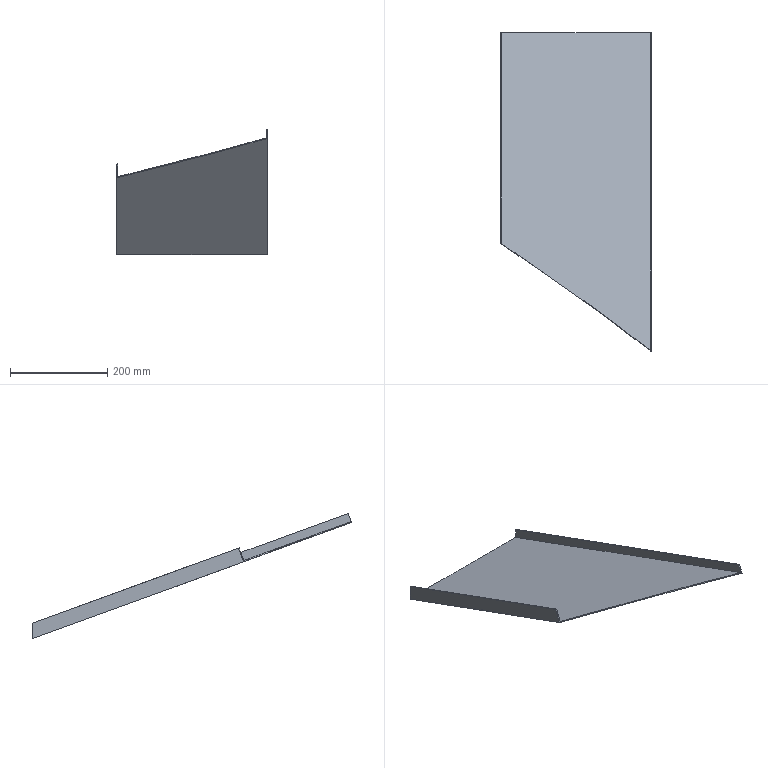Part | NX | features solid 2 | 1 solid | 11 faces | box 310 x 657.989 x 258.282 mm | volume 406239 mm3 | plane 10 | spline 1
STEP:
#1=CARTESIAN_POINT('',(513.,524.25,-139.857));
#2=VERTEX_POINT('',#1);
#3=CARTESIAN_POINT('',(513.,1180.,-378.53));
#4=VERTEX_POINT('',#3);
#5=CARTESIAN_POINT('',(513.,1053.844,-332.613));
#6=DIRECTION('',(0.,0.9397,-0.342));
#7=VECTOR('',#6,1000.);
#8=LINE('',#5,#7);
#9=EDGE_CURVE('',#2,#4,#8,.T.);
#10=ORIENTED_EDGE('',*,*,#9,.T.);
#11=CARTESIAN_POINT('',(207.,1180.,-378.53));
#12=VERTEX_POINT('',#11);
#13=CARTESIAN_POINT('',(-675.,1180.,-378.53));
#14=DIRECTION('',(-1.,0.,0.));
#15=VECTOR('',#14,1000.);
#16=LINE('',#13,#15);
#17=EDGE_CURVE('',#12,#4,#16,.F.);
#18=ORIENTED_EDGE('',*,*,#17,.F.);
#19=CARTESIAN_POINT('',(207.,744.184,-219.906));
#20=VERTEX_POINT('',#19);
#21=CARTESIAN_POINT('',(207.,1053.844,-332.613));
#22=DIRECTION('',(0.,0.9397,-0.342));
#23=VECTOR('',#22,1000.);
#24=LINE('',#21,#23);
#25=EDGE_CURVE('',#20,#12,#24,.T.);
#26=ORIENTED_EDGE('',*,*,#25,.F.);
#27=CARTESIAN_POINT('',(270.,700.581,-204.036));
#28=VERTEX_POINT('',#27);
#29=CARTESIAN_POINT('',(202.195,747.51,-221.116));
#30=CARTESIAN_POINT('',(270.081,700.526,-204.015));
#31=CARTESIAN_POINT('',(337.967,653.541,-186.914));
#32=CARTESIAN_POINT('',(342.606,650.33,-185.746));
#33=CARTESIAN_POINT('',(357.056,640.2,-182.059));
#34=CARTESIAN_POINT('',(366.847,633.337,-179.561));
#35=CARTESIAN_POINT('',(376.081,626.783,-177.175));
#36=CARTESIAN_POINT('',(395.621,612.917,-172.128));
#37=CARTESIAN_POINT('',(413.842,599.597,-167.281));
#38=CARTESIAN_POINT('',(451.399,572.143,-157.288));
#39=CARTESIAN_POINT('',(488.058,543.642,-146.914));
#40=CARTESIAN_POINT('',(518.274,520.15,-138.364));
#41=CARTESIAN_POINT('',(548.491,496.657,-129.813));
#42=CARTESIAN_POINT('',(578.708,473.165,-121.263));
#43=CARTESIAN_POINT('',(608.924,449.673,-112.712));
#44=CARTESIAN_POINT('',(639.141,426.18,-104.162));
#45=CARTESIAN_POINT('',(669.357,402.688,-95.611));
#46=CARTESIAN_POINT('',(699.574,379.196,-87.061));
#47=CARTESIAN_POINT('',(729.79,355.703,-78.51));
#48=B_SPLINE_CURVE_WITH_KNOTS('',2,(#29,#30,#31,#32,#33,#34,#35,#36,#37,#38,#39,#40,#41,#42,#43,#44,#45,#46,#47),.UNSPECIFIED.,.F.,.F.,(3,2,2,2,2,2,2,2,2,3),(-1.829,0.,0.125,0.25,0.5,1.,1.412,1.824,2.236,2.649),.PIECEWISE_BEZIER_KNOTS.);
#49=EDGE_CURVE('',#20,#28,#48,.T.);
#50=ORIENTED_EDGE('',*,*,#49,.T.);
#51=CARTESIAN_POINT('',(513.,524.25,-139.857));
#52=CARTESIAN_POINT('',(503.143,531.914,-142.646));
#53=CARTESIAN_POINT('',(483.463,547.283,-148.24));
#54=CARTESIAN_POINT('',(443.791,577.659,-159.296));
#55=CARTESIAN_POINT('',(393.431,614.763,-172.801));
#56=CARTESIAN_POINT('',(331.874,657.869,-188.49));
#57=CARTESIAN_POINT('',(290.605,686.32,-198.845));
#58=CARTESIAN_POINT('',(270.,700.581,-204.036));
#59=B_SPLINE_CURVE_WITH_KNOTS('',3,(#51,#52,#53,#54,#55,#56,#57,#58),.UNSPECIFIED.,.F.,.F.,(4,1,1,1,1,4),(0.525,0.5634,0.6018,0.6786,0.7553,0.8321),.UNSPECIFIED.);
#60=EDGE_CURVE('',#28,#2,#59,.F.);
#61=ORIENTED_EDGE('',*,*,#60,.T.);
#62=EDGE_LOOP('',(#10,#18,#26,#50,#61));
#63=FACE_BOUND('',#62,.T.);
#64=CARTESIAN_POINT('',(920.,1053.844,-332.613));
#65=DIRECTION('',(0.,0.342,0.9397));
#66=DIRECTION('',(0.,-0.9397,0.342));
#67=AXIS2_PLACEMENT_3D('',#64,#65,#66);
#68=PLANE('',#67);
#69=ADVANCED_FACE('',(#63),#68,.T.);
#70=CARTESIAN_POINT('',(205.,744.885,-222.289));
#71=VERTEX_POINT('',#70);
#72=CARTESIAN_POINT('',(205.,1180.,-380.658));
#73=VERTEX_POINT('',#72);
#74=CARTESIAN_POINT('',(205.,991.87,-312.185));
#75=DIRECTION('',(0.,0.9397,-0.342));
#76=VECTOR('',#75,1000.);
#77=LINE('',#74,#76);
#78=EDGE_CURVE('',#71,#73,#77,.T.);
#79=ORIENTED_EDGE('',*,*,#78,.F.);
#80=CARTESIAN_POINT('',(205.,755.145,-194.098));
#81=VERTEX_POINT('',#80);
#82=CARTESIAN_POINT('',(205.,755.145,-194.098));
#83=DIRECTION('',(0.,-0.342,-0.9397));
#84=VECTOR('',#83,1000.);
#85=LINE('',#82,#84);
#86=EDGE_CURVE('',#81,#71,#85,.T.);
#87=ORIENTED_EDGE('',*,*,#86,.F.);
#88=CARTESIAN_POINT('',(205.,1180.,-348.733));
#89=VERTEX_POINT('',#88);
#90=CARTESIAN_POINT('',(205.,1002.131,-283.994));
#91=DIRECTION('',(0.,-0.9397,0.342));
#92=VECTOR('',#91,1000.);
#93=LINE('',#90,#92);
#94=EDGE_CURVE('',#81,#89,#93,.F.);
#95=ORIENTED_EDGE('',*,*,#94,.T.);
#96=CARTESIAN_POINT('',(205.,1180.,-730.));
#97=DIRECTION('',(0.,0.,-1.));
#98=VECTOR('',#97,1000.);
#99=LINE('',#96,#98);
#100=EDGE_CURVE('',#73,#89,#99,.F.);
#101=ORIENTED_EDGE('',*,*,#100,.F.);
#102=EDGE_LOOP('',(#79,#87,#95,#101));
#103=FACE_BOUND('',#102,.T.);
#104=CARTESIAN_POINT('',(205.,999.395,-291.511));
#105=DIRECTION('',(-1.,0.,0.));
#106=DIRECTION('',(0.,-1.,0.));
#107=AXIS2_PLACEMENT_3D('',#104,#105,#106);
#108=PLANE('',#107);
#109=ADVANCED_FACE('',(#103),#108,.T.);
#110=CARTESIAN_POINT('',(513.,523.566,-141.736));
#111=VERTEX_POINT('',#110);
#112=CARTESIAN_POINT('',(513.,523.566,-141.736));
#113=CARTESIAN_POINT('',(500.551,533.245,-145.259));
#114=CARTESIAN_POINT('',(475.704,552.661,-152.326));
#115=CARTESIAN_POINT('',(425.39,590.785,-166.202));
#116=CARTESIAN_POINT('',(374.104,627.774,-179.665));
#117=CARTESIAN_POINT('',(322.106,663.848,-192.794));
#118=CARTESIAN_POINT('',(270.051,699.855,-205.9));
#119=CARTESIAN_POINT('',(231.022,726.875,-215.734));
#120=CARTESIAN_POINT('',(205.,744.885,-222.289));
#121=B_SPLINE_CURVE_WITH_KNOTS('',3,(#112,#113,#114,#115,#116,#117,#118,#119,#120),.UNSPECIFIED.,.F.,.F.,(4,1,1,1,1,1,4),(1.817,1.865,1.914,2.01,2.059,2.107,2.204),.UNSPECIFIED.);
#122=EDGE_CURVE('',#71,#111,#121,.F.);
#123=ORIENTED_EDGE('',*,*,#122,.F.);
#124=ORIENTED_EDGE('',*,*,#78,.T.);
#125=CARTESIAN_POINT('',(515.,1180.,-380.658));
#126=VERTEX_POINT('',#125);
#127=CARTESIAN_POINT('',(-675.,1180.,-380.658));
#128=DIRECTION('',(-1.,0.,0.));
#129=VECTOR('',#128,1000.);
#130=LINE('',#127,#129);
#131=EDGE_CURVE('',#73,#126,#130,.F.);
#132=ORIENTED_EDGE('',*,*,#131,.T.);
#133=CARTESIAN_POINT('',(515.,522.011,-141.17));
#134=VERTEX_POINT('',#133);
#135=CARTESIAN_POINT('',(515.,1053.16,-334.492));
#136=DIRECTION('',(0.,0.9397,-0.342));
#137=VECTOR('',#136,1000.);
#138=LINE('',#135,#137);
#139=EDGE_CURVE('',#134,#126,#138,.T.);
#140=ORIENTED_EDGE('',*,*,#139,.F.);
#141=CARTESIAN_POINT('',(513.,522.011,-141.17));
#142=VERTEX_POINT('',#141);
#143=CARTESIAN_POINT('',(515.,522.011,-141.17));
#144=DIRECTION('',(-1.,0.,0.));
#145=VECTOR('',#144,1000.);
#146=LINE('',#143,#145);
#147=EDGE_CURVE('',#134,#142,#146,.T.);
#148=ORIENTED_EDGE('',*,*,#147,.T.);
#149=CARTESIAN_POINT('',(513.,522.011,-141.17));
#150=DIRECTION('',(0.,0.9397,-0.342));
#151=VECTOR('',#150,1000.);
#152=LINE('',#149,#151);
#153=EDGE_CURVE('',#142,#111,#152,.T.);
#154=ORIENTED_EDGE('',*,*,#153,.T.);
#155=EDGE_LOOP('',(#123,#124,#132,#140,#148,#154));
#156=FACE_BOUND('',#155,.T.);
#157=CARTESIAN_POINT('',(920.,1053.16,-334.492));
#158=DIRECTION('',(0.,0.342,0.9397));
#159=DIRECTION('',(0.,-0.9397,0.342));
#160=AXIS2_PLACEMENT_3D('',#157,#158,#159);
#161=PLANE('',#160);
#162=ADVANCED_FACE('',(#156),#161,.F.);
#163=ORIENTED_EDGE('',*,*,#94,.F.);
#164=CARTESIAN_POINT('',(207.,753.761,-193.595));
#165=VERTEX_POINT('',#164);
#166=CARTESIAN_POINT('',(207.,753.761,-193.595));
#167=CARTESIAN_POINT('',(206.333,754.222,-193.763));
#168=CARTESIAN_POINT('',(205.667,754.684,-193.931));
#169=CARTESIAN_POINT('',(205.,755.145,-194.098));
#170=B_SPLINE_CURVE_WITH_KNOTS('',3,(#166,#167,#168,#169),.UNSPECIFIED.,.F.,.F.,(4,4),(0.07824,0.08073),.UNSPECIFIED.);
#171=EDGE_CURVE('',#165,#81,#170,.T.);
#172=ORIENTED_EDGE('',*,*,#171,.F.);
#173=CARTESIAN_POINT('',(207.,1180.,-348.733));
#174=VERTEX_POINT('',#173);
#175=CARTESIAN_POINT('',(207.,710.158,-177.724));
#176=DIRECTION('',(0.,-0.9397,0.342));
#177=VECTOR('',#176,1000.);
#178=LINE('',#175,#177);
#179=EDGE_CURVE('',#165,#174,#178,.F.);
#180=ORIENTED_EDGE('',*,*,#179,.T.);
#181=CARTESIAN_POINT('',(-675.,1180.,-348.733));
#182=DIRECTION('',(1.,0.,0.));
#183=VECTOR('',#182,1000.);
#184=LINE('',#181,#183);
#185=EDGE_CURVE('',#89,#174,#184,.T.);
#186=ORIENTED_EDGE('',*,*,#185,.F.);
#187=EDGE_LOOP('',(#163,#172,#180,#186));
#188=FACE_BOUND('',#187,.T.);
#189=CARTESIAN_POINT('',(270.,710.158,-177.724));
#190=DIRECTION('',(0.,-0.342,-0.9397));
#191=DIRECTION('',(0.,0.9397,-0.342));
#192=AXIS2_PLACEMENT_3D('',#189,#190,#191);
#193=PLANE('',#192);
#194=ADVANCED_FACE('',(#188),#193,.F.);
#195=ORIENTED_EDGE('',*,*,#25,.T.);
#196=CARTESIAN_POINT('',(207.,1180.,-730.));
#197=DIRECTION('',(0.,0.,1.));
#198=VECTOR('',#197,1000.);
#199=LINE('',#196,#198);
#200=EDGE_CURVE('',#174,#12,#199,.F.);
#201=ORIENTED_EDGE('',*,*,#200,.F.);
#202=ORIENTED_EDGE('',*,*,#179,.F.);
#203=CARTESIAN_POINT('',(207.,748.973,-206.75));
#204=DIRECTION('',(0.,-0.342,-0.9397));
#205=VECTOR('',#204,1000.);
#206=LINE('',#203,#205);
#207=EDGE_CURVE('',#20,#165,#206,.F.);
#208=ORIENTED_EDGE('',*,*,#207,.F.);
#209=EDGE_LOOP('',(#195,#201,#202,#208));
#210=FACE_BOUND('',#209,.T.);
#211=CARTESIAN_POINT('',(207.,706.738,-187.121));
#212=DIRECTION('',(1.,0.,0.));
#213=DIRECTION('',(0.,1.,0.));
#214=AXIS2_PLACEMENT_3D('',#211,#212,#213);
#215=PLANE('',#214);
#216=ADVANCED_FACE('',(#210),#215,.T.);
#217=ORIENTED_EDGE('',*,*,#60,.F.);
#218=ORIENTED_EDGE('',*,*,#49,.F.);
#219=ORIENTED_EDGE('',*,*,#207,.T.);
#220=ORIENTED_EDGE('',*,*,#171,.T.);
#221=ORIENTED_EDGE('',*,*,#86,.T.);
#222=ORIENTED_EDGE('',*,*,#122,.T.);
#223=CARTESIAN_POINT('',(513.,531.091,-121.063));
#224=DIRECTION('',(0.,-0.342,-0.9397));
#225=VECTOR('',#224,1000.);
#226=LINE('',#223,#225);
#227=EDGE_CURVE('',#2,#111,#226,.T.);
#228=ORIENTED_EDGE('',*,*,#227,.F.);
#229=EDGE_LOOP('',(#217,#218,#219,#220,#221,#222,#228));
#230=FACE_BOUND('',#229,.T.);
#231=CARTESIAN_POINT('',(205.,755.145,-194.098));
#232=CARTESIAN_POINT('',(205.,744.885,-222.289));
#233=CARTESIAN_POINT('',(223.318,742.467,-189.484));
#234=CARTESIAN_POINT('',(223.318,732.206,-217.675));
#235=CARTESIAN_POINT('',(246.217,726.619,-183.716));
#236=CARTESIAN_POINT('',(246.217,716.358,-211.906));
#237=CARTESIAN_POINT('',(273.694,707.601,-176.794));
#238=CARTESIAN_POINT('',(273.694,697.341,-204.985));
#239=CARTESIAN_POINT('',(287.433,698.092,-173.333));
#240=CARTESIAN_POINT('',(287.433,687.832,-201.524));
#241=CARTESIAN_POINT('',(298.882,690.168,-170.449));
#242=CARTESIAN_POINT('',(298.882,679.908,-198.64));
#243=CARTESIAN_POINT('',(308.042,683.829,-168.141));
#244=CARTESIAN_POINT('',(308.042,673.568,-196.332));
#245=CARTESIAN_POINT('',(314.911,679.075,-166.411));
#246=CARTESIAN_POINT('',(314.911,668.814,-194.602));
#247=CARTESIAN_POINT('',(321.781,674.32,-164.68));
#248=CARTESIAN_POINT('',(321.781,664.06,-192.871));
#249=CARTESIAN_POINT('',(327.504,670.359,-163.239));
#250=CARTESIAN_POINT('',(327.504,660.098,-191.429));
#251=CARTESIAN_POINT('',(332.085,667.188,-162.085));
#252=CARTESIAN_POINT('',(332.085,656.927,-190.275));
#253=CARTESIAN_POINT('',(334.944,665.209,-161.364));
#254=CARTESIAN_POINT('',(334.944,654.949,-189.555));
#255=CARTESIAN_POINT('',(337.241,663.62,-160.786));
#256=CARTESIAN_POINT('',(337.241,653.359,-188.977));
#257=CARTESIAN_POINT('',(338.938,662.445,-160.358));
#258=CARTESIAN_POINT('',(338.938,652.185,-188.549));
#259=CARTESIAN_POINT('',(341.397,660.734,-159.736));
#260=CARTESIAN_POINT('',(341.397,650.473,-187.926));
#261=CARTESIAN_POINT('',(344.504,658.565,-158.946));
#262=CARTESIAN_POINT('',(344.504,648.304,-187.137));
#263=CARTESIAN_POINT('',(348.288,655.919,-157.983));
#264=CARTESIAN_POINT('',(348.288,645.659,-186.174));
#265=CARTESIAN_POINT('',(352.007,653.315,-157.035));
#266=CARTESIAN_POINT('',(352.007,643.055,-185.226));
#267=CARTESIAN_POINT('',(354.685,651.439,-156.352));
#268=CARTESIAN_POINT('',(354.685,641.178,-184.543));
#269=CARTESIAN_POINT('',(355.986,650.527,-156.02));
#270=CARTESIAN_POINT('',(355.986,640.266,-184.211));
#271=CARTESIAN_POINT('',(356.517,650.154,-155.885));
#272=CARTESIAN_POINT('',(356.517,639.894,-184.076));
#273=CARTESIAN_POINT('',(356.994,649.821,-155.763));
#274=CARTESIAN_POINT('',(356.994,639.56,-183.954));
#275=CARTESIAN_POINT('',(357.305,649.602,-155.684));
#276=CARTESIAN_POINT('',(357.305,639.342,-183.875));
#277=CARTESIAN_POINT('',(357.827,649.236,-155.551));
#278=CARTESIAN_POINT('',(357.827,638.976,-183.741));
#279=CARTESIAN_POINT('',(358.583,648.706,-155.358));
#280=CARTESIAN_POINT('',(358.583,638.445,-183.548));
#281=CARTESIAN_POINT('',(359.783,647.864,-155.051));
#282=CARTESIAN_POINT('',(359.783,637.603,-183.242));
#283=CARTESIAN_POINT('',(361.279,646.813,-154.669));
#284=CARTESIAN_POINT('',(361.279,636.552,-182.859));
#285=CARTESIAN_POINT('',(363.064,645.558,-154.212));
#286=CARTESIAN_POINT('',(363.064,635.297,-182.403));
#287=CARTESIAN_POINT('',(365.432,643.891,-153.605));
#288=CARTESIAN_POINT('',(365.432,633.63,-181.796));
#289=CARTESIAN_POINT('',(368.365,641.823,-152.852));
#290=CARTESIAN_POINT('',(368.365,631.562,-181.043));
#291=CARTESIAN_POINT('',(371.86,639.352,-151.953));
#292=CARTESIAN_POINT('',(371.86,629.092,-180.144));
#293=CARTESIAN_POINT('',(374.698,637.341,-151.221));
#294=CARTESIAN_POINT('',(374.698,627.081,-179.412));
#295=CARTESIAN_POINT('',(377.045,635.676,-150.615));
#296=CARTESIAN_POINT('',(377.045,625.415,-178.806));
#297=CARTESIAN_POINT('',(379.464,633.957,-149.99));
#298=CARTESIAN_POINT('',(379.464,623.697,-178.18));
#299=CARTESIAN_POINT('',(383.64,630.984,-148.907));
#300=CARTESIAN_POINT('',(383.64,620.723,-177.098));
#301=CARTESIAN_POINT('',(389.569,626.746,-147.365));
#302=CARTESIAN_POINT('',(389.569,616.485,-175.556));
#303=CARTESIAN_POINT('',(396.586,621.702,-145.529));
#304=CARTESIAN_POINT('',(396.586,611.441,-173.72));
#305=CARTESIAN_POINT('',(403.507,616.701,-143.709));
#306=CARTESIAN_POINT('',(403.507,606.44,-171.899));
#307=CARTESIAN_POINT('',(409.227,612.544,-142.196));
#308=CARTESIAN_POINT('',(409.227,602.283,-170.387));
#309=CARTESIAN_POINT('',(413.694,609.283,-141.009));
#310=CARTESIAN_POINT('',(413.694,599.022,-169.2));
#311=CARTESIAN_POINT('',(418.36,605.868,-139.766));
#312=CARTESIAN_POINT('',(418.36,595.607,-167.957));
#313=CARTESIAN_POINT('',(424.124,601.631,-138.224));
#314=CARTESIAN_POINT('',(424.124,591.37,-166.414));
#315=CARTESIAN_POINT('',(437.974,591.39,-134.496));
#316=CARTESIAN_POINT('',(437.974,581.129,-162.687));
#317=CARTESIAN_POINT('',(458.619,575.914,-128.864));
#318=CARTESIAN_POINT('',(458.619,565.653,-157.054));
#319=CARTESIAN_POINT('',(485.887,554.958,-121.236));
#320=CARTESIAN_POINT('',(485.887,544.698,-149.427));
#321=CARTESIAN_POINT('',(503.953,540.86,-116.105));
#322=CARTESIAN_POINT('',(503.953,530.6,-144.296));
#323=CARTESIAN_POINT('',(513.,533.827,-113.545));
#324=CARTESIAN_POINT('',(513.,523.566,-141.736));
#325=B_SPLINE_SURFACE_WITH_KNOTS('',3,1,((#231,#232),(#233,#234),(#235,#236),(#237,#238),(#239,#240),(#241,#242),(#243,#244),(#245,#246),(#247,#248),(#249,#250),(#251,#252),(#253,#254),(#255,#256),(#257,#258),(#259,#260),(#261,#262),(#263,#264),(#265,#266),(#267,#268),(#269,#270),(#271,#272),(#273,#274),(#275,#276),(#277,#278),(#279,#280),(#281,#282),(#283,#284),(#285,#286),(#287,#288),(#289,#290),(#291,#292),(#293,#294),(#295,#296),(#297,#298),(#299,#300),(#301,#302),(#303,#304),(#305,#306),(#307,#308),(#309,#310),(#311,#312),(#313,#314),(#315,#316),(#317,#318),(#319,#320),(#321,#322),(#323,#324)),.UNSPECIFIED.,.F.,.F.,.F.,(4,1,1,1,1,1,1,1,1,1,1,1,1,1,1,1,1,1,1,1,1,1,1,1,1,1,1,1,1,1,1,1,1,1,1,1,1,1,1,1,1,1,1,1,4),(2,2),(-1.791,-1.051,-0.8659,-0.6808,-0.4957,-0.4031,-0.3106,-0.2181,-0.1255,-0.07924,-0.03297,-0.009836,0.0133,0.03644,0.05957,0.08271,0.1058,0.1174,0.1203,0.1232,0.1246,0.1261,0.129,0.1348,0.1405,0.1521,0.1637,0.1753,0.1984,0.2215,0.2447,0.2562,0.2678,0.2909,0.3372,0.3835,0.4297,0.476,0.4992,0.5223,0.5686,0.6148,0.7999,0.985,1.17),(0.,1.),.UNSPECIFIED.);
#326=ADVANCED_FACE('',(#230),#325,.F.);
#327=ORIENTED_EDGE('',*,*,#17,.T.);
#328=CARTESIAN_POINT('',(513.,1180.,-359.375));
#329=VERTEX_POINT('',#328);
#330=CARTESIAN_POINT('',(513.,1180.,-730.));
#331=DIRECTION('',(0.,0.,-1.));
#332=VECTOR('',#331,1000.);
#333=LINE('',#330,#332);
#334=EDGE_CURVE('',#4,#329,#333,.F.);
#335=ORIENTED_EDGE('',*,*,#334,.T.);
#336=CARTESIAN_POINT('',(515.,1180.,-359.375));
#337=VERTEX_POINT('',#336);
#338=CARTESIAN_POINT('',(515.,1180.,-359.375));
#339=DIRECTION('',(-1.,0.,0.));
#340=VECTOR('',#339,1000.);
#341=LINE('',#338,#340);
#342=EDGE_CURVE('',#337,#329,#341,.T.);
#343=ORIENTED_EDGE('',*,*,#342,.F.);
#344=CARTESIAN_POINT('',(515.,1180.,-730.));
#345=DIRECTION('',(0.,0.,-1.));
#346=VECTOR('',#345,1000.);
#347=LINE('',#344,#346);
#348=EDGE_CURVE('',#126,#337,#347,.F.);
#349=ORIENTED_EDGE('',*,*,#348,.F.);
#350=ORIENTED_EDGE('',*,*,#131,.F.);
#351=ORIENTED_EDGE('',*,*,#100,.T.);
#352=ORIENTED_EDGE('',*,*,#185,.T.);
#353=ORIENTED_EDGE('',*,*,#200,.T.);
#354=EDGE_LOOP('',(#327,#335,#343,#349,#350,#351,#352,#353));
#355=FACE_BOUND('',#354,.T.);
#356=CARTESIAN_POINT('',(-675.,1180.,-730.));
#357=DIRECTION('',(0.,-1.,0.));
#358=DIRECTION('',(1.,0.,0.));
#359=AXIS2_PLACEMENT_3D('',#356,#357,#358);
#360=PLANE('',#359);
#361=ADVANCED_FACE('',(#355),#360,.F.);
#362=CARTESIAN_POINT('',(515.,528.852,-122.376));
#363=VERTEX_POINT('',#362);
#364=CARTESIAN_POINT('',(515.,522.353,-140.23));
#365=DIRECTION('',(0.,-0.342,-0.9397));
#366=VECTOR('',#365,1000.);
#367=LINE('',#364,#366);
#368=EDGE_CURVE('',#363,#134,#367,.T.);
#369=ORIENTED_EDGE('',*,*,#368,.T.);
#370=ORIENTED_EDGE('',*,*,#139,.T.);
#371=ORIENTED_EDGE('',*,*,#348,.T.);
#372=CARTESIAN_POINT('',(515.,528.852,-122.376));
#373=DIRECTION('',(0.,0.9397,-0.342));
#374=VECTOR('',#373,1000.);
#375=LINE('',#372,#374);
#376=EDGE_CURVE('',#363,#337,#375,.T.);
#377=ORIENTED_EDGE('',*,*,#376,.F.);
#378=EDGE_LOOP('',(#369,#370,#371,#377));
#379=FACE_BOUND('',#378,.T.);
#380=CARTESIAN_POINT('',(515.,985.,-145.));
#381=DIRECTION('',(-1.,0.,0.));
#382=DIRECTION('',(0.,0.,-1.));
#383=AXIS2_PLACEMENT_3D('',#380,#381,#382);
#384=PLANE('',#383);
#385=ADVANCED_FACE('',(#379),#384,.F.);
#386=ORIENTED_EDGE('',*,*,#227,.T.);
#387=ORIENTED_EDGE('',*,*,#153,.F.);
#388=CARTESIAN_POINT('',(513.,528.852,-122.376));
#389=VERTEX_POINT('',#388);
#390=CARTESIAN_POINT('',(513.,522.011,-141.17));
#391=DIRECTION('',(0.,0.342,0.9397));
#392=VECTOR('',#391,1000.);
#393=LINE('',#390,#392);
#394=EDGE_CURVE('',#142,#389,#393,.T.);
#395=ORIENTED_EDGE('',*,*,#394,.T.);
#396=CARTESIAN_POINT('',(513.,528.852,-122.376));
#397=DIRECTION('',(0.,0.9397,-0.342));
#398=VECTOR('',#397,1000.);
#399=LINE('',#396,#398);
#400=EDGE_CURVE('',#389,#329,#399,.T.);
#401=ORIENTED_EDGE('',*,*,#400,.T.);
#402=ORIENTED_EDGE('',*,*,#334,.F.);
#403=ORIENTED_EDGE('',*,*,#9,.F.);
#404=EDGE_LOOP('',(#386,#387,#395,#401,#402,#403));
#405=FACE_BOUND('',#404,.T.);
#406=CARTESIAN_POINT('',(513.,522.011,-141.17));
#407=DIRECTION('',(-1.,0.,0.));
#408=DIRECTION('',(0.,0.,-1.));
#409=AXIS2_PLACEMENT_3D('',#406,#407,#408);
#410=PLANE('',#409);
#411=ADVANCED_FACE('',(#405),#410,.T.);
#412=ORIENTED_EDGE('',*,*,#342,.T.);
#413=ORIENTED_EDGE('',*,*,#400,.F.);
#414=CARTESIAN_POINT('',(515.,528.852,-122.376));
#415=DIRECTION('',(-1.,0.,0.));
#416=VECTOR('',#415,1000.);
#417=LINE('',#414,#416);
#418=EDGE_CURVE('',#363,#389,#417,.T.);
#419=ORIENTED_EDGE('',*,*,#418,.F.);
#420=ORIENTED_EDGE('',*,*,#376,.T.);
#421=EDGE_LOOP('',(#412,#413,#419,#420));
#422=FACE_BOUND('',#421,.T.);
#423=CARTESIAN_POINT('',(515.,528.852,-122.376));
#424=DIRECTION('',(0.,-0.342,-0.9397));
#425=DIRECTION('',(0.,0.9397,-0.342));
#426=AXIS2_PLACEMENT_3D('',#423,#424,#425);
#427=PLANE('',#426);
#428=ADVANCED_FACE('',(#422),#427,.F.);
#429=ORIENTED_EDGE('',*,*,#368,.F.);
#430=ORIENTED_EDGE('',*,*,#418,.T.);
#431=ORIENTED_EDGE('',*,*,#394,.F.);
#432=ORIENTED_EDGE('',*,*,#147,.F.);
#433=EDGE_LOOP('',(#429,#430,#431,#432));
#434=FACE_BOUND('',#433,.T.);
#435=CARTESIAN_POINT('',(515.,522.011,-141.17));
#436=DIRECTION('',(0.,0.9397,-0.342));
#437=DIRECTION('',(0.,0.342,0.9397));
#438=AXIS2_PLACEMENT_3D('',#435,#436,#437);
#439=PLANE('',#438);
#440=ADVANCED_FACE('',(#434),#439,.F.);
#441=CLOSED_SHELL('',(#69,#109,#162,#194,#216,#326,#361,#385,#411,#428,#440));
#442=MANIFOLD_SOLID_BREP('',#441);
#443=(LENGTH_UNIT()NAMED_UNIT(*)SI_UNIT(.MILLI.,.METRE.));
#444=UNCERTAINTY_MEASURE_WITH_UNIT(LENGTH_MEASURE(0.0508),#443,'','');
#445=(NAMED_UNIT(*)PLANE_ANGLE_UNIT()SI_UNIT($,.RADIAN.));
#446=(NAMED_UNIT(*)SI_UNIT($,.STERADIAN.)SOLID_ANGLE_UNIT());
#447=(GEOMETRIC_REPRESENTATION_CONTEXT(3)GLOBAL_UNCERTAINTY_ASSIGNED_CONTEXT((#444))GLOBAL_UNIT_ASSIGNED_CONTEXT((#443,#445,#446))REPRESENTATION_CONTEXT('',''));
#448=ADVANCED_BREP_SHAPE_REPRESENTATION('',(#442),#447);